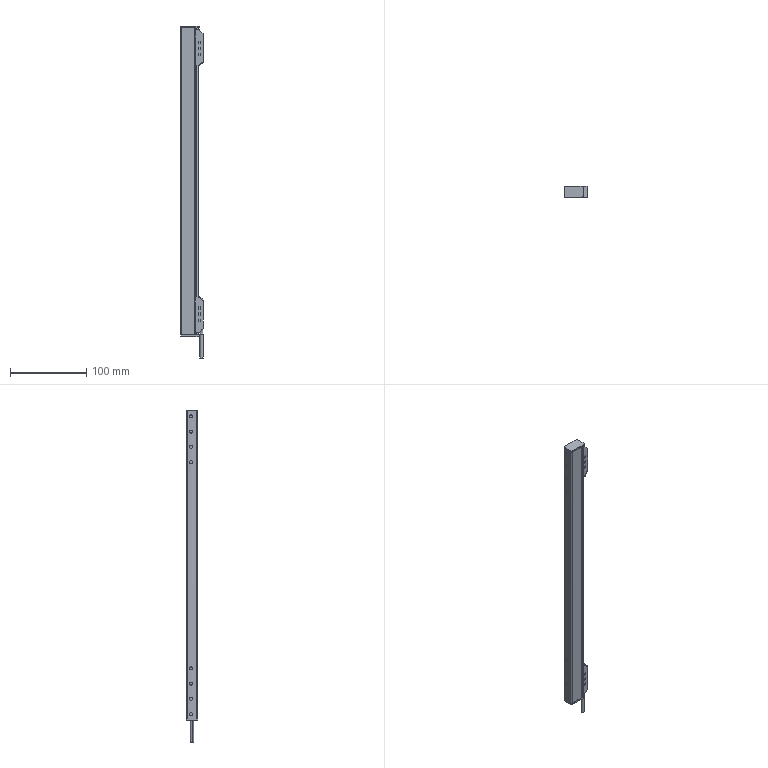Part | SolidWorks | features BaseBody 1 | 1 solid | 222 faces | box 30 x 14.8 x 434.725 mm | volume 136537 mm3 | plane 143 | cylinder 77 | spline 2 | commonest cylinder face diameters 2 x59 3 x12 1 x2 4 x2 10 x2